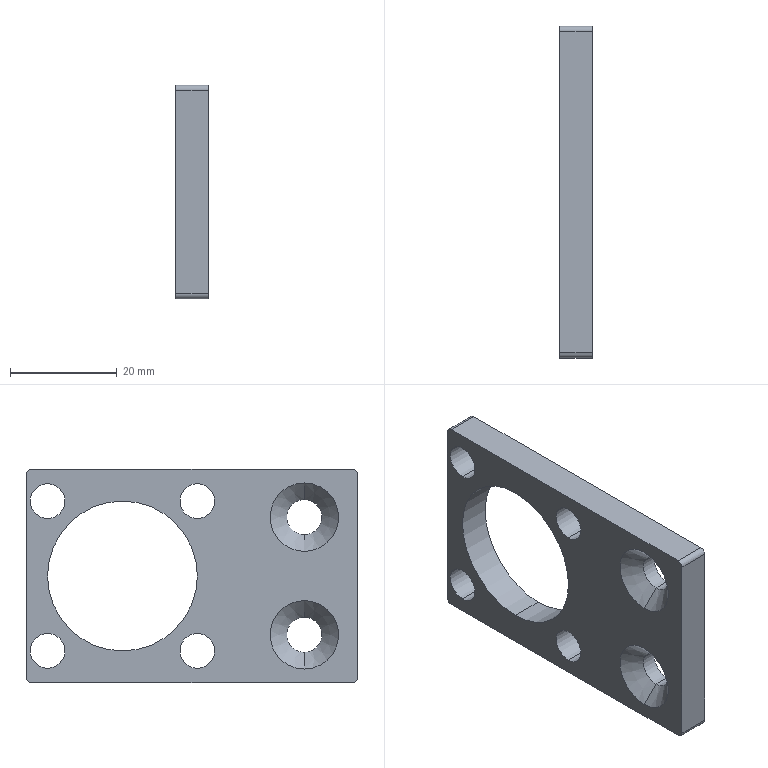Part | SolidWorks | features BaseBody 1 | 1 solid | 28 faces | box 6 x 62 x 40 mm | volume 9712 mm3 | cylinder 18 | plane 6 | cone 4 | commonest cylinder face diameters 6.5 x8 2 x4 6.6 x4 28 x2
STEP:
#1=CARTESIAN_POINT('',(6.,13.,14.));
#2=VERTEX_POINT('',#1);
#3=CARTESIAN_POINT('',(6.,13.,-14.));
#4=VERTEX_POINT('',#3);
#5=CARTESIAN_POINT('',(6.,13.,0.));
#6=DIRECTION('',(1.,0.,0.));
#7=DIRECTION('',(0.,0.,1.));
#8=AXIS2_PLACEMENT_3D('',#5,#6,#7);
#9=CIRCLE('',#8,14.);
#10=EDGE_CURVE('',#2,#4,#9,.T.);
#11=ORIENTED_EDGE('',*,*,#10,.T.);
#12=CARTESIAN_POINT('',(0.,13.,-14.));
#13=VERTEX_POINT('',#12);
#14=CARTESIAN_POINT('',(10.,13.,-14.));
#15=DIRECTION('',(-1.,0.,0.));
#16=VECTOR('',#15,1000.);
#17=LINE('',#14,#16);
#18=EDGE_CURVE('',#4,#13,#17,.T.);
#19=ORIENTED_EDGE('',*,*,#18,.T.);
#20=CARTESIAN_POINT('',(0.,13.,14.));
#21=VERTEX_POINT('',#20);
#22=CARTESIAN_POINT('',(0.,13.,0.));
#23=DIRECTION('',(1.,0.,0.));
#24=DIRECTION('',(0.,0.,1.));
#25=AXIS2_PLACEMENT_3D('',#22,#23,#24);
#26=CIRCLE('',#25,14.);
#27=EDGE_CURVE('',#21,#13,#26,.T.);
#28=ORIENTED_EDGE('',*,*,#27,.F.);
#29=CARTESIAN_POINT('',(10.,13.,14.));
#30=DIRECTION('',(-1.,0.,0.));
#31=VECTOR('',#30,1000.);
#32=LINE('',#29,#31);
#33=EDGE_CURVE('',#2,#21,#32,.T.);
#34=ORIENTED_EDGE('',*,*,#33,.F.);
#35=EDGE_LOOP('',(#11,#19,#28,#34));
#36=FACE_OUTER_BOUND('',#35,.T.);
#37=CARTESIAN_POINT('',(10.,13.,0.));
#38=DIRECTION('',(-1.,0.,0.));
#39=DIRECTION('',(0.,0.,1.));
#40=AXIS2_PLACEMENT_3D('',#37,#38,#39);
#41=CYLINDRICAL_SURFACE('',#40,14.);
#42=ADVANCED_FACE('',(#36),#41,.F.);
#43=CARTESIAN_POINT('',(6.,27.,-10.75));
#44=VERTEX_POINT('',#43);
#45=CARTESIAN_POINT('',(6.,27.,-17.25));
#46=VERTEX_POINT('',#45);
#47=CARTESIAN_POINT('',(6.,27.,-14.));
#48=DIRECTION('',(1.,0.,0.));
#49=DIRECTION('',(0.,0.,1.));
#50=AXIS2_PLACEMENT_3D('',#47,#48,#49);
#51=CIRCLE('',#50,3.25);
#52=EDGE_CURVE('',#44,#46,#51,.T.);
#53=ORIENTED_EDGE('',*,*,#52,.T.);
#54=CARTESIAN_POINT('',(0.,27.,-17.25));
#55=VERTEX_POINT('',#54);
#56=CARTESIAN_POINT('',(10.,27.,-17.25));
#57=DIRECTION('',(-1.,0.,0.));
#58=VECTOR('',#57,1000.);
#59=LINE('',#56,#58);
#60=EDGE_CURVE('',#46,#55,#59,.T.);
#61=ORIENTED_EDGE('',*,*,#60,.T.);
#62=CARTESIAN_POINT('',(0.,27.,-10.75));
#63=VERTEX_POINT('',#62);
#64=CARTESIAN_POINT('',(0.,27.,-14.));
#65=DIRECTION('',(1.,0.,0.));
#66=DIRECTION('',(0.,0.,1.));
#67=AXIS2_PLACEMENT_3D('',#64,#65,#66);
#68=CIRCLE('',#67,3.25);
#69=EDGE_CURVE('',#63,#55,#68,.T.);
#70=ORIENTED_EDGE('',*,*,#69,.F.);
#71=CARTESIAN_POINT('',(10.,27.,-10.75));
#72=DIRECTION('',(-1.,0.,0.));
#73=VECTOR('',#72,1000.);
#74=LINE('',#71,#73);
#75=EDGE_CURVE('',#44,#63,#74,.T.);
#76=ORIENTED_EDGE('',*,*,#75,.F.);
#77=EDGE_LOOP('',(#53,#61,#70,#76));
#78=FACE_OUTER_BOUND('',#77,.T.);
#79=CARTESIAN_POINT('',(10.,27.,-14.));
#80=DIRECTION('',(-1.,0.,0.));
#81=DIRECTION('',(0.,0.,1.));
#82=AXIS2_PLACEMENT_3D('',#79,#80,#81);
#83=CYLINDRICAL_SURFACE('',#82,3.25);
#84=ADVANCED_FACE('',(#78),#83,.F.);
#85=CARTESIAN_POINT('',(6.,-1.,-10.75));
#86=VERTEX_POINT('',#85);
#87=CARTESIAN_POINT('',(6.,-1.,-17.25));
#88=VERTEX_POINT('',#87);
#89=CARTESIAN_POINT('',(6.,-1.,-14.));
#90=DIRECTION('',(1.,0.,0.));
#91=DIRECTION('',(0.,0.,1.));
#92=AXIS2_PLACEMENT_3D('',#89,#90,#91);
#93=CIRCLE('',#92,3.25);
#94=EDGE_CURVE('',#86,#88,#93,.T.);
#95=ORIENTED_EDGE('',*,*,#94,.T.);
#96=CARTESIAN_POINT('',(0.,-1.,-17.25));
#97=VERTEX_POINT('',#96);
#98=CARTESIAN_POINT('',(10.,-1.,-17.25));
#99=DIRECTION('',(-1.,0.,0.));
#100=VECTOR('',#99,1000.);
#101=LINE('',#98,#100);
#102=EDGE_CURVE('',#88,#97,#101,.T.);
#103=ORIENTED_EDGE('',*,*,#102,.T.);
#104=CARTESIAN_POINT('',(0.,-1.,-10.75));
#105=VERTEX_POINT('',#104);
#106=CARTESIAN_POINT('',(0.,-1.,-14.));
#107=DIRECTION('',(1.,0.,0.));
#108=DIRECTION('',(0.,0.,1.));
#109=AXIS2_PLACEMENT_3D('',#106,#107,#108);
#110=CIRCLE('',#109,3.25);
#111=EDGE_CURVE('',#105,#97,#110,.T.);
#112=ORIENTED_EDGE('',*,*,#111,.F.);
#113=CARTESIAN_POINT('',(10.,-1.,-10.75));
#114=DIRECTION('',(-1.,0.,0.));
#115=VECTOR('',#114,1000.);
#116=LINE('',#113,#115);
#117=EDGE_CURVE('',#86,#105,#116,.T.);
#118=ORIENTED_EDGE('',*,*,#117,.F.);
#119=EDGE_LOOP('',(#95,#103,#112,#118));
#120=FACE_OUTER_BOUND('',#119,.T.);
#121=CARTESIAN_POINT('',(10.,-1.,-14.));
#122=DIRECTION('',(-1.,0.,0.));
#123=DIRECTION('',(0.,0.,1.));
#124=AXIS2_PLACEMENT_3D('',#121,#122,#123);
#125=CYLINDRICAL_SURFACE('',#124,3.25);
#126=ADVANCED_FACE('',(#120),#125,.F.);
#127=CARTESIAN_POINT('',(6.,-1.,17.25));
#128=VERTEX_POINT('',#127);
#129=CARTESIAN_POINT('',(6.,-1.,10.75));
#130=VERTEX_POINT('',#129);
#131=CARTESIAN_POINT('',(6.,-1.,14.));
#132=DIRECTION('',(1.,0.,0.));
#133=DIRECTION('',(0.,0.,1.));
#134=AXIS2_PLACEMENT_3D('',#131,#132,#133);
#135=CIRCLE('',#134,3.25);
#136=EDGE_CURVE('',#128,#130,#135,.T.);
#137=ORIENTED_EDGE('',*,*,#136,.T.);
#138=CARTESIAN_POINT('',(0.,-1.,10.75));
#139=VERTEX_POINT('',#138);
#140=CARTESIAN_POINT('',(10.,-1.,10.75));
#141=DIRECTION('',(-1.,0.,0.));
#142=VECTOR('',#141,1000.);
#143=LINE('',#140,#142);
#144=EDGE_CURVE('',#130,#139,#143,.T.);
#145=ORIENTED_EDGE('',*,*,#144,.T.);
#146=CARTESIAN_POINT('',(0.,-1.,17.25));
#147=VERTEX_POINT('',#146);
#148=CARTESIAN_POINT('',(0.,-1.,14.));
#149=DIRECTION('',(1.,0.,0.));
#150=DIRECTION('',(0.,0.,1.));
#151=AXIS2_PLACEMENT_3D('',#148,#149,#150);
#152=CIRCLE('',#151,3.25);
#153=EDGE_CURVE('',#147,#139,#152,.T.);
#154=ORIENTED_EDGE('',*,*,#153,.F.);
#155=CARTESIAN_POINT('',(10.,-1.,17.25));
#156=DIRECTION('',(-1.,0.,0.));
#157=VECTOR('',#156,1000.);
#158=LINE('',#155,#157);
#159=EDGE_CURVE('',#128,#147,#158,.T.);
#160=ORIENTED_EDGE('',*,*,#159,.F.);
#161=EDGE_LOOP('',(#137,#145,#154,#160));
#162=FACE_OUTER_BOUND('',#161,.T.);
#163=CARTESIAN_POINT('',(10.,-1.,14.));
#164=DIRECTION('',(-1.,0.,0.));
#165=DIRECTION('',(0.,0.,1.));
#166=AXIS2_PLACEMENT_3D('',#163,#164,#165);
#167=CYLINDRICAL_SURFACE('',#166,3.25);
#168=ADVANCED_FACE('',(#162),#167,.F.);
#169=CARTESIAN_POINT('',(6.,27.,17.25));
#170=VERTEX_POINT('',#169);
#171=CARTESIAN_POINT('',(6.,27.,10.75));
#172=VERTEX_POINT('',#171);
#173=CARTESIAN_POINT('',(6.,27.,14.));
#174=DIRECTION('',(1.,0.,0.));
#175=DIRECTION('',(0.,0.,1.));
#176=AXIS2_PLACEMENT_3D('',#173,#174,#175);
#177=CIRCLE('',#176,3.25);
#178=EDGE_CURVE('',#170,#172,#177,.T.);
#179=ORIENTED_EDGE('',*,*,#178,.T.);
#180=CARTESIAN_POINT('',(0.,27.,10.75));
#181=VERTEX_POINT('',#180);
#182=CARTESIAN_POINT('',(10.,27.,10.75));
#183=DIRECTION('',(-1.,0.,0.));
#184=VECTOR('',#183,1000.);
#185=LINE('',#182,#184);
#186=EDGE_CURVE('',#172,#181,#185,.T.);
#187=ORIENTED_EDGE('',*,*,#186,.T.);
#188=CARTESIAN_POINT('',(0.,27.,17.25));
#189=VERTEX_POINT('',#188);
#190=CARTESIAN_POINT('',(0.,27.,14.));
#191=DIRECTION('',(1.,0.,0.));
#192=DIRECTION('',(0.,0.,1.));
#193=AXIS2_PLACEMENT_3D('',#190,#191,#192);
#194=CIRCLE('',#193,3.25);
#195=EDGE_CURVE('',#189,#181,#194,.T.);
#196=ORIENTED_EDGE('',*,*,#195,.F.);
#197=CARTESIAN_POINT('',(10.,27.,17.25));
#198=DIRECTION('',(-1.,0.,0.));
#199=VECTOR('',#198,1000.);
#200=LINE('',#197,#199);
#201=EDGE_CURVE('',#170,#189,#200,.T.);
#202=ORIENTED_EDGE('',*,*,#201,.F.);
#203=EDGE_LOOP('',(#179,#187,#196,#202));
#204=FACE_OUTER_BOUND('',#203,.T.);
#205=CARTESIAN_POINT('',(10.,27.,14.));
#206=DIRECTION('',(-1.,0.,0.));
#207=DIRECTION('',(0.,0.,1.));
#208=AXIS2_PLACEMENT_3D('',#205,#206,#207);
#209=CYLINDRICAL_SURFACE('',#208,3.25);
#210=ADVANCED_FACE('',(#204),#209,.F.);
#211=CARTESIAN_POINT('',(6.,-21.,14.3));
#212=VERTEX_POINT('',#211);
#213=CARTESIAN_POINT('',(6.,-21.,7.7));
#214=VERTEX_POINT('',#213);
#215=CARTESIAN_POINT('',(6.,-21.,11.));
#216=DIRECTION('',(1.,0.,0.));
#217=DIRECTION('',(0.,0.,1.));
#218=AXIS2_PLACEMENT_3D('',#215,#216,#217);
#219=CIRCLE('',#218,3.3);
#220=EDGE_CURVE('',#212,#214,#219,.T.);
#221=ORIENTED_EDGE('',*,*,#220,.T.);
#222=CARTESIAN_POINT('',(3.1,-21.,7.7));
#223=VERTEX_POINT('',#222);
#224=CARTESIAN_POINT('',(0.,-21.,7.7));
#225=DIRECTION('',(-1.,0.,0.));
#226=VECTOR('',#225,1000.);
#227=LINE('',#224,#226);
#228=EDGE_CURVE('',#214,#223,#227,.T.);
#229=ORIENTED_EDGE('',*,*,#228,.T.);
#230=CARTESIAN_POINT('',(3.1,-21.,14.3));
#231=VERTEX_POINT('',#230);
#232=CARTESIAN_POINT('',(3.1,-21.,11.));
#233=DIRECTION('',(1.,0.,0.));
#234=DIRECTION('',(0.,0.,1.));
#235=AXIS2_PLACEMENT_3D('',#232,#233,#234);
#236=CIRCLE('',#235,3.3);
#237=EDGE_CURVE('',#231,#223,#236,.T.);
#238=ORIENTED_EDGE('',*,*,#237,.F.);
#239=CARTESIAN_POINT('',(0.,-21.,14.3));
#240=DIRECTION('',(-1.,0.,0.));
#241=VECTOR('',#240,1000.);
#242=LINE('',#239,#241);
#243=EDGE_CURVE('',#212,#231,#242,.T.);
#244=ORIENTED_EDGE('',*,*,#243,.F.);
#245=EDGE_LOOP('',(#221,#229,#238,#244));
#246=FACE_OUTER_BOUND('',#245,.T.);
#247=CARTESIAN_POINT('',(0.,-21.,11.));
#248=DIRECTION('',(-1.,0.,0.));
#249=DIRECTION('',(0.,0.,1.));
#250=AXIS2_PLACEMENT_3D('',#247,#248,#249);
#251=CYLINDRICAL_SURFACE('',#250,3.3);
#252=ADVANCED_FACE('',(#246),#251,.F.);
#253=CARTESIAN_POINT('',(6.,-21.,-7.7));
#254=VERTEX_POINT('',#253);
#255=CARTESIAN_POINT('',(6.,-21.,-14.3));
#256=VERTEX_POINT('',#255);
#257=CARTESIAN_POINT('',(6.,-21.,-11.));
#258=DIRECTION('',(1.,0.,0.));
#259=DIRECTION('',(0.,0.,1.));
#260=AXIS2_PLACEMENT_3D('',#257,#258,#259);
#261=CIRCLE('',#260,3.3);
#262=EDGE_CURVE('',#254,#256,#261,.T.);
#263=ORIENTED_EDGE('',*,*,#262,.T.);
#264=CARTESIAN_POINT('',(3.1,-21.,-14.3));
#265=VERTEX_POINT('',#264);
#266=CARTESIAN_POINT('',(0.,-21.,-14.3));
#267=DIRECTION('',(-1.,0.,0.));
#268=VECTOR('',#267,1000.);
#269=LINE('',#266,#268);
#270=EDGE_CURVE('',#256,#265,#269,.T.);
#271=ORIENTED_EDGE('',*,*,#270,.T.);
#272=CARTESIAN_POINT('',(3.1,-21.,-7.7));
#273=VERTEX_POINT('',#272);
#274=CARTESIAN_POINT('',(3.1,-21.,-11.));
#275=DIRECTION('',(1.,0.,0.));
#276=DIRECTION('',(0.,0.,1.));
#277=AXIS2_PLACEMENT_3D('',#274,#275,#276);
#278=CIRCLE('',#277,3.3);
#279=EDGE_CURVE('',#273,#265,#278,.T.);
#280=ORIENTED_EDGE('',*,*,#279,.F.);
#281=CARTESIAN_POINT('',(0.,-21.,-7.7));
#282=DIRECTION('',(-1.,0.,0.));
#283=VECTOR('',#282,1000.);
#284=LINE('',#281,#283);
#285=EDGE_CURVE('',#254,#273,#284,.T.);
#286=ORIENTED_EDGE('',*,*,#285,.F.);
#287=EDGE_LOOP('',(#263,#271,#280,#286));
#288=FACE_OUTER_BOUND('',#287,.T.);
#289=CARTESIAN_POINT('',(0.,-21.,-11.));
#290=DIRECTION('',(-1.,0.,0.));
#291=DIRECTION('',(0.,0.,1.));
#292=AXIS2_PLACEMENT_3D('',#289,#290,#291);
#293=CYLINDRICAL_SURFACE('',#292,3.3);
#294=ADVANCED_FACE('',(#288),#293,.F.);
#295=ORIENTED_EDGE('',*,*,#237,.T.);
#296=CARTESIAN_POINT('',(0.,-21.,4.6));
#297=VERTEX_POINT('',#296);
#298=CARTESIAN_POINT('',(0.,-21.,4.6));
#299=DIRECTION('',(-0.7071,0.,-0.7071));
#300=VECTOR('',#299,1000.);
#301=LINE('',#298,#300);
#302=EDGE_CURVE('',#223,#297,#301,.T.);
#303=ORIENTED_EDGE('',*,*,#302,.T.);
#304=CARTESIAN_POINT('',(0.,-21.,17.4));
#305=VERTEX_POINT('',#304);
#306=CARTESIAN_POINT('',(0.,-21.,11.));
#307=DIRECTION('',(1.,0.,0.));
#308=DIRECTION('',(0.,0.,1.));
#309=AXIS2_PLACEMENT_3D('',#306,#307,#308);
#310=CIRCLE('',#309,6.4);
#311=EDGE_CURVE('',#305,#297,#310,.T.);
#312=ORIENTED_EDGE('',*,*,#311,.F.);
#313=CARTESIAN_POINT('',(0.,-21.,17.4));
#314=DIRECTION('',(-0.7071,0.,0.7071));
#315=VECTOR('',#314,1000.);
#316=LINE('',#313,#315);
#317=EDGE_CURVE('',#231,#305,#316,.T.);
#318=ORIENTED_EDGE('',*,*,#317,.F.);
#319=EDGE_LOOP('',(#295,#303,#312,#318));
#320=FACE_OUTER_BOUND('',#319,.T.);
#321=CARTESIAN_POINT('',(0.,-21.,11.));
#322=DIRECTION('',(-1.,0.,0.));
#323=DIRECTION('',(0.,0.,1.));
#324=AXIS2_PLACEMENT_3D('',#321,#322,#323);
#325=CONICAL_SURFACE('',#324,6.4,0.7854);
#326=ADVANCED_FACE('',(#320),#325,.F.);
#327=ORIENTED_EDGE('',*,*,#279,.T.);
#328=CARTESIAN_POINT('',(0.,-21.,-17.4));
#329=VERTEX_POINT('',#328);
#330=CARTESIAN_POINT('',(0.,-21.,-17.4));
#331=DIRECTION('',(-0.7071,0.,-0.7071));
#332=VECTOR('',#331,1000.);
#333=LINE('',#330,#332);
#334=EDGE_CURVE('',#265,#329,#333,.T.);
#335=ORIENTED_EDGE('',*,*,#334,.T.);
#336=CARTESIAN_POINT('',(0.,-21.,-4.6));
#337=VERTEX_POINT('',#336);
#338=CARTESIAN_POINT('',(0.,-21.,-11.));
#339=DIRECTION('',(1.,0.,0.));
#340=DIRECTION('',(0.,0.,1.));
#341=AXIS2_PLACEMENT_3D('',#338,#339,#340);
#342=CIRCLE('',#341,6.4);
#343=EDGE_CURVE('',#337,#329,#342,.T.);
#344=ORIENTED_EDGE('',*,*,#343,.F.);
#345=CARTESIAN_POINT('',(0.,-21.,-4.6));
#346=DIRECTION('',(-0.7071,0.,0.7071));
#347=VECTOR('',#346,1000.);
#348=LINE('',#345,#347);
#349=EDGE_CURVE('',#273,#337,#348,.T.);
#350=ORIENTED_EDGE('',*,*,#349,.F.);
#351=EDGE_LOOP('',(#327,#335,#344,#350));
#352=FACE_OUTER_BOUND('',#351,.T.);
#353=CARTESIAN_POINT('',(0.,-21.,-11.));
#354=DIRECTION('',(-1.,0.,0.));
#355=DIRECTION('',(0.,0.,1.));
#356=AXIS2_PLACEMENT_3D('',#353,#354,#355);
#357=CONICAL_SURFACE('',#356,6.4,0.7854);
#358=ADVANCED_FACE('',(#352),#357,.F.);
#359=CARTESIAN_POINT('',(6.,-30.,-20.));
#360=VERTEX_POINT('',#359);
#361=CARTESIAN_POINT('',(6.,-31.,-19.));
#362=VERTEX_POINT('',#361);
#363=CARTESIAN_POINT('',(6.,-30.,-19.));
#364=DIRECTION('',(-1.,0.,0.));
#365=DIRECTION('',(0.,0.,1.));
#366=AXIS2_PLACEMENT_3D('',#363,#364,#365);
#367=CIRCLE('',#366,1.);
#368=EDGE_CURVE('',#360,#362,#367,.T.);
#369=ORIENTED_EDGE('',*,*,#368,.F.);
#370=CARTESIAN_POINT('',(6.,30.,-20.));
#371=VERTEX_POINT('',#370);
#372=CARTESIAN_POINT('',(6.,0.,-20.));
#373=DIRECTION('',(0.,-1.,0.));
#374=VECTOR('',#373,1000.);
#375=LINE('',#372,#374);
#376=EDGE_CURVE('',#371,#360,#375,.T.);
#377=ORIENTED_EDGE('',*,*,#376,.F.);
#378=CARTESIAN_POINT('',(6.,31.,-19.));
#379=VERTEX_POINT('',#378);
#380=CARTESIAN_POINT('',(6.,30.,-19.));
#381=DIRECTION('',(-1.,0.,0.));
#382=DIRECTION('',(0.,0.,1.));
#383=AXIS2_PLACEMENT_3D('',#380,#381,#382);
#384=CIRCLE('',#383,1.);
#385=EDGE_CURVE('',#379,#371,#384,.T.);
#386=ORIENTED_EDGE('',*,*,#385,.F.);
#387=CARTESIAN_POINT('',(6.,31.,19.));
#388=VERTEX_POINT('',#387);
#389=CARTESIAN_POINT('',(6.,31.,0.));
#390=DIRECTION('',(0.,0.,-1.));
#391=VECTOR('',#390,1000.);
#392=LINE('',#389,#391);
#393=EDGE_CURVE('',#388,#379,#392,.T.);
#394=ORIENTED_EDGE('',*,*,#393,.F.);
#395=CARTESIAN_POINT('',(6.,30.,20.));
#396=VERTEX_POINT('',#395);
#397=CARTESIAN_POINT('',(6.,30.,19.));
#398=DIRECTION('',(-1.,0.,0.));
#399=DIRECTION('',(0.,0.,1.));
#400=AXIS2_PLACEMENT_3D('',#397,#398,#399);
#401=CIRCLE('',#400,1.);
#402=EDGE_CURVE('',#396,#388,#401,.T.);
#403=ORIENTED_EDGE('',*,*,#402,.F.);
#404=CARTESIAN_POINT('',(6.,-30.,20.));
#405=VERTEX_POINT('',#404);
#406=CARTESIAN_POINT('',(6.,0.,20.));
#407=DIRECTION('',(0.,1.,0.));
#408=VECTOR('',#407,1000.);
#409=LINE('',#406,#408);
#410=EDGE_CURVE('',#405,#396,#409,.T.);
#411=ORIENTED_EDGE('',*,*,#410,.F.);
#412=CARTESIAN_POINT('',(6.,-31.,19.));
#413=VERTEX_POINT('',#412);
#414=CARTESIAN_POINT('',(6.,-30.,19.));
#415=DIRECTION('',(-1.,0.,0.));
#416=DIRECTION('',(0.,0.,1.));
#417=AXIS2_PLACEMENT_3D('',#414,#415,#416);
#418=CIRCLE('',#417,1.);
#419=EDGE_CURVE('',#413,#405,#418,.T.);
#420=ORIENTED_EDGE('',*,*,#419,.F.);
#421=CARTESIAN_POINT('',(6.,-31.,0.));
#422=DIRECTION('',(0.,0.,1.));
#423=VECTOR('',#422,1000.);
#424=LINE('',#421,#423);
#425=EDGE_CURVE('',#362,#413,#424,.T.);
#426=ORIENTED_EDGE('',*,*,#425,.F.);
#427=EDGE_LOOP('',(#369,#377,#386,#394,#403,#411,#420,#426));
#428=FACE_OUTER_BOUND('',#427,.T.);
#429=ORIENTED_EDGE('',*,*,#10,.F.);
#430=CARTESIAN_POINT('',(6.,13.,0.));
#431=DIRECTION('',(1.,0.,0.));
#432=DIRECTION('',(0.,0.,1.));
#433=AXIS2_PLACEMENT_3D('',#430,#431,#432);
#434=CIRCLE('',#433,14.);
#435=EDGE_CURVE('',#4,#2,#434,.T.);
#436=ORIENTED_EDGE('',*,*,#435,.F.);
#437=EDGE_LOOP('',(#429,#436));
#438=FACE_BOUND('',#437,.T.);
#439=ORIENTED_EDGE('',*,*,#52,.F.);
#440=CARTESIAN_POINT('',(6.,27.,-14.));
#441=DIRECTION('',(1.,0.,0.));
#442=DIRECTION('',(0.,0.,1.));
#443=AXIS2_PLACEMENT_3D('',#440,#441,#442);
#444=CIRCLE('',#443,3.25);
#445=EDGE_CURVE('',#46,#44,#444,.T.);
#446=ORIENTED_EDGE('',*,*,#445,.F.);
#447=EDGE_LOOP('',(#439,#446));
#448=FACE_BOUND('',#447,.T.);
#449=ORIENTED_EDGE('',*,*,#94,.F.);
#450=CARTESIAN_POINT('',(6.,-1.,-14.));
#451=DIRECTION('',(1.,0.,0.));
#452=DIRECTION('',(0.,0.,1.));
#453=AXIS2_PLACEMENT_3D('',#450,#451,#452);
#454=CIRCLE('',#453,3.25);
#455=EDGE_CURVE('',#88,#86,#454,.T.);
#456=ORIENTED_EDGE('',*,*,#455,.F.);
#457=EDGE_LOOP('',(#449,#456));
#458=FACE_BOUND('',#457,.T.);
#459=ORIENTED_EDGE('',*,*,#136,.F.);
#460=CARTESIAN_POINT('',(6.,-1.,14.));
#461=DIRECTION('',(1.,0.,0.));
#462=DIRECTION('',(0.,0.,1.));
#463=AXIS2_PLACEMENT_3D('',#460,#461,#462);
#464=CIRCLE('',#463,3.25);
#465=EDGE_CURVE('',#130,#128,#464,.T.);
#466=ORIENTED_EDGE('',*,*,#465,.F.);
#467=EDGE_LOOP('',(#459,#466));
#468=FACE_BOUND('',#467,.T.);
#469=ORIENTED_EDGE('',*,*,#178,.F.);
#470=CARTESIAN_POINT('',(6.,27.,14.));
#471=DIRECTION('',(1.,0.,0.));
#472=DIRECTION('',(0.,0.,1.));
#473=AXIS2_PLACEMENT_3D('',#470,#471,#472);
#474=CIRCLE('',#473,3.25);
#475=EDGE_CURVE('',#172,#170,#474,.T.);
#476=ORIENTED_EDGE('',*,*,#475,.F.);
#477=EDGE_LOOP('',(#469,#476));
#478=FACE_BOUND('',#477,.T.);
#479=ORIENTED_EDGE('',*,*,#220,.F.);
#480=CARTESIAN_POINT('',(6.,-21.,11.));
#481=DIRECTION('',(1.,0.,0.));
#482=DIRECTION('',(0.,0.,1.));
#483=AXIS2_PLACEMENT_3D('',#480,#481,#482);
#484=CIRCLE('',#483,3.3);
#485=EDGE_CURVE('',#214,#212,#484,.T.);
#486=ORIENTED_EDGE('',*,*,#485,.F.);
#487=EDGE_LOOP('',(#479,#486));
#488=FACE_BOUND('',#487,.T.);
#489=ORIENTED_EDGE('',*,*,#262,.F.);
#490=CARTESIAN_POINT('',(6.,-21.,-11.));
#491=DIRECTION('',(1.,0.,0.));
#492=DIRECTION('',(0.,0.,1.));
#493=AXIS2_PLACEMENT_3D('',#490,#491,#492);
#494=CIRCLE('',#493,3.3);
#495=EDGE_CURVE('',#256,#254,#494,.T.);
#496=ORIENTED_EDGE('',*,*,#495,.F.);
#497=EDGE_LOOP('',(#489,#496));
#498=FACE_BOUND('',#497,.T.);
#499=CARTESIAN_POINT('',(6.,0.,0.));
#500=DIRECTION('',(-1.,0.,0.));
#501=DIRECTION('',(0.,0.,1.));
#502=AXIS2_PLACEMENT_3D('',#499,#500,#501);
#503=PLANE('',#502);
#504=ADVANCED_FACE('',(#428,#438,#448,#458,#468,#478,#488,#498),#503,.F.);
#505=CARTESIAN_POINT('',(0.,-31.,-19.));
#506=VERTEX_POINT('',#505);
#507=CARTESIAN_POINT('',(6.,-31.,-19.));
#508=DIRECTION('',(-1.,0.,0.));
#509=VECTOR('',#508,1000.);
#510=LINE('',#507,#509);
#511=EDGE_CURVE('',#362,#506,#510,.T.);
#512=ORIENTED_EDGE('',*,*,#511,.F.);
#513=ORIENTED_EDGE('',*,*,#425,.T.);
#514=CARTESIAN_POINT('',(0.,-31.,19.));
#515=VERTEX_POINT('',#514);
#516=CARTESIAN_POINT('',(6.,-31.,19.));
#517=DIRECTION('',(1.,0.,0.));
#518=VECTOR('',#517,1000.);
#519=LINE('',#516,#518);
#520=EDGE_CURVE('',#515,#413,#519,.T.);
#521=ORIENTED_EDGE('',*,*,#520,.F.);
#522=CARTESIAN_POINT('',(0.,-31.,20.));
#523=DIRECTION('',(0.,0.,1.));
#524=VECTOR('',#523,1000.);
#525=LINE('',#522,#524);
#526=EDGE_CURVE('',#506,#515,#525,.T.);
#527=ORIENTED_EDGE('',*,*,#526,.F.);
#528=EDGE_LOOP('',(#512,#513,#521,#527));
#529=FACE_OUTER_BOUND('',#528,.T.);
#530=CARTESIAN_POINT('',(6.,-31.,20.));
#531=DIRECTION('',(0.,1.,0.));
#532=DIRECTION('',(0.,0.,1.));
#533=AXIS2_PLACEMENT_3D('',#530,#531,#532);
#534=PLANE('',#533);
#535=ADVANCED_FACE('',(#529),#534,.F.);
#536=CARTESIAN_POINT('',(0.,-30.,-20.));
#537=VERTEX_POINT('',#536);
#538=CARTESIAN_POINT('',(6.,-30.,-20.));
#539=DIRECTION('',(1.,0.,0.));
#540=VECTOR('',#539,1000.);
#541=LINE('',#538,#540);
#542=EDGE_CURVE('',#537,#360,#541,.T.);
#543=ORIENTED_EDGE('',*,*,#542,.F.);
#544=CARTESIAN_POINT('',(0.,30.,-20.));
#545=VERTEX_POINT('',#544);
#546=CARTESIAN_POINT('',(0.,-31.,-20.));
#547=DIRECTION('',(0.,-1.,0.));
#548=VECTOR('',#547,1000.);
#549=LINE('',#546,#548);
#550=EDGE_CURVE('',#545,#537,#549,.T.);
#551=ORIENTED_EDGE('',*,*,#550,.F.);
#552=CARTESIAN_POINT('',(6.,30.,-20.));
#553=DIRECTION('',(-1.,0.,0.));
#554=VECTOR('',#553,1000.);
#555=LINE('',#552,#554);
#556=EDGE_CURVE('',#371,#545,#555,.T.);
#557=ORIENTED_EDGE('',*,*,#556,.F.);
#558=ORIENTED_EDGE('',*,*,#376,.T.);
#559=EDGE_LOOP('',(#543,#551,#557,#558));
#560=FACE_OUTER_BOUND('',#559,.T.);
#561=CARTESIAN_POINT('',(6.,-31.,-20.));
#562=DIRECTION('',(0.,0.,1.));
#563=DIRECTION('',(1.,0.,0.));
#564=AXIS2_PLACEMENT_3D('',#561,#562,#563);
#565=PLANE('',#564);
#566=ADVANCED_FACE('',(#560),#565,.F.);
#567=CARTESIAN_POINT('',(0.,31.,-19.));
#568=VERTEX_POINT('',#567);
#569=CARTESIAN_POINT('',(6.,31.,-19.));
#570=DIRECTION('',(1.,0.,0.));
#571=VECTOR('',#570,1000.);
#572=LINE('',#569,#571);
#573=EDGE_CURVE('',#568,#379,#572,.T.);
#574=ORIENTED_EDGE('',*,*,#573,.F.);
#575=CARTESIAN_POINT('',(0.,31.,19.));
#576=VERTEX_POINT('',#575);
#577=CARTESIAN_POINT('',(0.,31.,20.));
#578=DIRECTION('',(0.,0.,-1.));
#579=VECTOR('',#578,1000.);
#580=LINE('',#577,#579);
#581=EDGE_CURVE('',#576,#568,#580,.T.);
#582=ORIENTED_EDGE('',*,*,#581,.F.);
#583=CARTESIAN_POINT('',(6.,31.,19.));
#584=DIRECTION('',(-1.,0.,0.));
#585=VECTOR('',#584,1000.);
#586=LINE('',#583,#585);
#587=EDGE_CURVE('',#388,#576,#586,.T.);
#588=ORIENTED_EDGE('',*,*,#587,.F.);
#589=ORIENTED_EDGE('',*,*,#393,.T.);
#590=EDGE_LOOP('',(#574,#582,#588,#589));
#591=FACE_OUTER_BOUND('',#590,.T.);
#592=CARTESIAN_POINT('',(6.,31.,20.));
#593=DIRECTION('',(0.,-1.,0.));
#594=DIRECTION('',(0.,0.,-1.));
#595=AXIS2_PLACEMENT_3D('',#592,#593,#594);
#596=PLANE('',#595);
#597=ADVANCED_FACE('',(#591),#596,.F.);
#598=CARTESIAN_POINT('',(0.,-30.,20.));
#599=VERTEX_POINT('',#598);
#600=CARTESIAN_POINT('',(6.,-30.,20.));
#601=DIRECTION('',(-1.,0.,0.));
#602=VECTOR('',#601,1000.);
#603=LINE('',#600,#602);
#604=EDGE_CURVE('',#405,#599,#603,.T.);
#605=ORIENTED_EDGE('',*,*,#604,.F.);
#606=ORIENTED_EDGE('',*,*,#410,.T.);
#607=CARTESIAN_POINT('',(0.,30.,20.));
#608=VERTEX_POINT('',#607);
#609=CARTESIAN_POINT('',(6.,30.,20.));
#610=DIRECTION('',(1.,0.,0.));
#611=VECTOR('',#610,1000.);
#612=LINE('',#609,#611);
#613=EDGE_CURVE('',#608,#396,#612,.T.);
#614=ORIENTED_EDGE('',*,*,#613,.F.);
#615=CARTESIAN_POINT('',(0.,-31.,20.));
#616=DIRECTION('',(0.,1.,0.));
#617=VECTOR('',#616,1000.);
#618=LINE('',#615,#617);
#619=EDGE_CURVE('',#599,#608,#618,.T.);
#620=ORIENTED_EDGE('',*,*,#619,.F.);
#621=EDGE_LOOP('',(#605,#606,#614,#620));
#622=FACE_OUTER_BOUND('',#621,.T.);
#623=CARTESIAN_POINT('',(6.,-31.,20.));
#624=DIRECTION('',(0.,0.,-1.));
#625=DIRECTION('',(-1.,0.,0.));
#626=AXIS2_PLACEMENT_3D('',#623,#624,#625);
#627=PLANE('',#626);
#628=ADVANCED_FACE('',(#622),#627,.F.);
#629=ORIENTED_EDGE('',*,*,#18,.F.);
#630=ORIENTED_EDGE('',*,*,#435,.T.);
#631=ORIENTED_EDGE('',*,*,#33,.T.);
#632=CARTESIAN_POINT('',(0.,13.,0.));
#633=DIRECTION('',(1.,0.,0.));
#634=DIRECTION('',(0.,0.,1.));
#635=AXIS2_PLACEMENT_3D('',#632,#633,#634);
#636=CIRCLE('',#635,14.);
#637=EDGE_CURVE('',#13,#21,#636,.T.);
#638=ORIENTED_EDGE('',*,*,#637,.F.);
#639=EDGE_LOOP('',(#629,#630,#631,#638));
#640=FACE_OUTER_BOUND('',#639,.T.);
#641=CARTESIAN_POINT('',(10.,13.,0.));
#642=DIRECTION('',(-1.,0.,0.));
#643=DIRECTION('',(0.,0.,1.));
#644=AXIS2_PLACEMENT_3D('',#641,#642,#643);
#645=CYLINDRICAL_SURFACE('',#644,14.);
#646=ADVANCED_FACE('',(#640),#645,.F.);
#647=ORIENTED_EDGE('',*,*,#60,.F.);
#648=ORIENTED_EDGE('',*,*,#445,.T.);
#649=ORIENTED_EDGE('',*,*,#75,.T.);
#650=CARTESIAN_POINT('',(0.,27.,-14.));
#651=DIRECTION('',(1.,0.,0.));
#652=DIRECTION('',(0.,0.,1.));
#653=AXIS2_PLACEMENT_3D('',#650,#651,#652);
#654=CIRCLE('',#653,3.25);
#655=EDGE_CURVE('',#55,#63,#654,.T.);
#656=ORIENTED_EDGE('',*,*,#655,.F.);
#657=EDGE_LOOP('',(#647,#648,#649,#656));
#658=FACE_OUTER_BOUND('',#657,.T.);
#659=CARTESIAN_POINT('',(10.,27.,-14.));
#660=DIRECTION('',(-1.,0.,0.));
#661=DIRECTION('',(0.,0.,1.));
#662=AXIS2_PLACEMENT_3D('',#659,#660,#661);
#663=CYLINDRICAL_SURFACE('',#662,3.25);
#664=ADVANCED_FACE('',(#658),#663,.F.);
#665=ORIENTED_EDGE('',*,*,#102,.F.);
#666=ORIENTED_EDGE('',*,*,#455,.T.);
#667=ORIENTED_EDGE('',*,*,#117,.T.);
#668=CARTESIAN_POINT('',(0.,-1.,-14.));
#669=DIRECTION('',(1.,0.,0.));
#670=DIRECTION('',(0.,0.,1.));
#671=AXIS2_PLACEMENT_3D('',#668,#669,#670);
#672=CIRCLE('',#671,3.25);
#673=EDGE_CURVE('',#97,#105,#672,.T.);
#674=ORIENTED_EDGE('',*,*,#673,.F.);
#675=EDGE_LOOP('',(#665,#666,#667,#674));
#676=FACE_OUTER_BOUND('',#675,.T.);
#677=CARTESIAN_POINT('',(10.,-1.,-14.));
#678=DIRECTION('',(-1.,0.,0.));
#679=DIRECTION('',(0.,0.,1.));
#680=AXIS2_PLACEMENT_3D('',#677,#678,#679);
#681=CYLINDRICAL_SURFACE('',#680,3.25);
#682=ADVANCED_FACE('',(#676),#681,.F.);
#683=ORIENTED_EDGE('',*,*,#144,.F.);
#684=ORIENTED_EDGE('',*,*,#465,.T.);
#685=ORIENTED_EDGE('',*,*,#159,.T.);
#686=CARTESIAN_POINT('',(0.,-1.,14.));
#687=DIRECTION('',(1.,0.,0.));
#688=DIRECTION('',(0.,0.,1.));
#689=AXIS2_PLACEMENT_3D('',#686,#687,#688);
#690=CIRCLE('',#689,3.25);
#691=EDGE_CURVE('',#139,#147,#690,.T.);
#692=ORIENTED_EDGE('',*,*,#691,.F.);
#693=EDGE_LOOP('',(#683,#684,#685,#692));
#694=FACE_OUTER_BOUND('',#693,.T.);
#695=CARTESIAN_POINT('',(10.,-1.,14.));
#696=DIRECTION('',(-1.,0.,0.));
#697=DIRECTION('',(0.,0.,1.));
#698=AXIS2_PLACEMENT_3D('',#695,#696,#697);
#699=CYLINDRICAL_SURFACE('',#698,3.25);
#700=ADVANCED_FACE('',(#694),#699,.F.);
#701=ORIENTED_EDGE('',*,*,#186,.F.);
#702=ORIENTED_EDGE('',*,*,#475,.T.);
#703=ORIENTED_EDGE('',*,*,#201,.T.);
#704=CARTESIAN_POINT('',(0.,27.,14.));
#705=DIRECTION('',(1.,0.,0.));
#706=DIRECTION('',(0.,0.,1.));
#707=AXIS2_PLACEMENT_3D('',#704,#705,#706);
#708=CIRCLE('',#707,3.25);
#709=EDGE_CURVE('',#181,#189,#708,.T.);
#710=ORIENTED_EDGE('',*,*,#709,.F.);
#711=EDGE_LOOP('',(#701,#702,#703,#710));
#712=FACE_OUTER_BOUND('',#711,.T.);
#713=CARTESIAN_POINT('',(10.,27.,14.));
#714=DIRECTION('',(-1.,0.,0.));
#715=DIRECTION('',(0.,0.,1.));
#716=AXIS2_PLACEMENT_3D('',#713,#714,#715);
#717=CYLINDRICAL_SURFACE('',#716,3.25);
#718=ADVANCED_FACE('',(#712),#717,.F.);
#719=ORIENTED_EDGE('',*,*,#228,.F.);
#720=ORIENTED_EDGE('',*,*,#485,.T.);
#721=ORIENTED_EDGE('',*,*,#243,.T.);
#722=CARTESIAN_POINT('',(3.1,-21.,11.));
#723=DIRECTION('',(1.,0.,0.));
#724=DIRECTION('',(0.,0.,1.));
#725=AXIS2_PLACEMENT_3D('',#722,#723,#724);
#726=CIRCLE('',#725,3.3);
#727=EDGE_CURVE('',#223,#231,#726,.T.);
#728=ORIENTED_EDGE('',*,*,#727,.F.);
#729=EDGE_LOOP('',(#719,#720,#721,#728));
#730=FACE_OUTER_BOUND('',#729,.T.);
#731=CARTESIAN_POINT('',(0.,-21.,11.));
#732=DIRECTION('',(-1.,0.,0.));
#733=DIRECTION('',(0.,0.,1.));
#734=AXIS2_PLACEMENT_3D('',#731,#732,#733);
#735=CYLINDRICAL_SURFACE('',#734,3.3);
#736=ADVANCED_FACE('',(#730),#735,.F.);
#737=ORIENTED_EDGE('',*,*,#270,.F.);
#738=ORIENTED_EDGE('',*,*,#495,.T.);
#739=ORIENTED_EDGE('',*,*,#285,.T.);
#740=CARTESIAN_POINT('',(3.1,-21.,-11.));
#741=DIRECTION('',(1.,0.,0.));
#742=DIRECTION('',(0.,0.,1.));
#743=AXIS2_PLACEMENT_3D('',#740,#741,#742);
#744=CIRCLE('',#743,3.3);
#745=EDGE_CURVE('',#265,#273,#744,.T.);
#746=ORIENTED_EDGE('',*,*,#745,.F.);
#747=EDGE_LOOP('',(#737,#738,#739,#746));
#748=FACE_OUTER_BOUND('',#747,.T.);
#749=CARTESIAN_POINT('',(0.,-21.,-11.));
#750=DIRECTION('',(-1.,0.,0.));
#751=DIRECTION('',(0.,0.,1.));
#752=AXIS2_PLACEMENT_3D('',#749,#750,#751);
#753=CYLINDRICAL_SURFACE('',#752,3.3);
#754=ADVANCED_FACE('',(#748),#753,.F.);
#755=ORIENTED_EDGE('',*,*,#581,.T.);
#756=CARTESIAN_POINT('',(0.,30.,-19.));
#757=DIRECTION('',(-1.,0.,0.));
#758=DIRECTION('',(0.,0.,1.));
#759=AXIS2_PLACEMENT_3D('',#756,#757,#758);
#760=CIRCLE('',#759,1.);
#761=EDGE_CURVE('',#568,#545,#760,.T.);
#762=ORIENTED_EDGE('',*,*,#761,.T.);
#763=ORIENTED_EDGE('',*,*,#550,.T.);
#764=CARTESIAN_POINT('',(0.,-30.,-19.));
#765=DIRECTION('',(-1.,0.,0.));
#766=DIRECTION('',(0.,0.,1.));
#767=AXIS2_PLACEMENT_3D('',#764,#765,#766);
#768=CIRCLE('',#767,1.);
#769=EDGE_CURVE('',#537,#506,#768,.T.);
#770=ORIENTED_EDGE('',*,*,#769,.T.);
#771=ORIENTED_EDGE('',*,*,#526,.T.);
#772=CARTESIAN_POINT('',(0.,-30.,19.));
#773=DIRECTION('',(-1.,0.,0.));
#774=DIRECTION('',(0.,0.,1.));
#775=AXIS2_PLACEMENT_3D('',#772,#773,#774);
#776=CIRCLE('',#775,1.);
#777=EDGE_CURVE('',#515,#599,#776,.T.);
#778=ORIENTED_EDGE('',*,*,#777,.T.);
#779=ORIENTED_EDGE('',*,*,#619,.T.);
#780=CARTESIAN_POINT('',(0.,30.,19.));
#781=DIRECTION('',(-1.,0.,0.));
#782=DIRECTION('',(0.,0.,1.));
#783=AXIS2_PLACEMENT_3D('',#780,#781,#782);
#784=CIRCLE('',#783,1.);
#785=EDGE_CURVE('',#608,#576,#784,.T.);
#786=ORIENTED_EDGE('',*,*,#785,.T.);
#787=EDGE_LOOP('',(#755,#762,#763,#770,#771,#778,#779,#786));
#788=FACE_OUTER_BOUND('',#787,.T.);
#789=ORIENTED_EDGE('',*,*,#27,.T.);
#790=ORIENTED_EDGE('',*,*,#637,.T.);
#791=EDGE_LOOP('',(#789,#790));
#792=FACE_BOUND('',#791,.T.);
#793=ORIENTED_EDGE('',*,*,#69,.T.);
#794=ORIENTED_EDGE('',*,*,#655,.T.);
#795=EDGE_LOOP('',(#793,#794));
#796=FACE_BOUND('',#795,.T.);
#797=ORIENTED_EDGE('',*,*,#111,.T.);
#798=ORIENTED_EDGE('',*,*,#673,.T.);
#799=EDGE_LOOP('',(#797,#798));
#800=FACE_BOUND('',#799,.T.);
#801=ORIENTED_EDGE('',*,*,#153,.T.);
#802=ORIENTED_EDGE('',*,*,#691,.T.);
#803=EDGE_LOOP('',(#801,#802));
#804=FACE_BOUND('',#803,.T.);
#805=ORIENTED_EDGE('',*,*,#195,.T.);
#806=ORIENTED_EDGE('',*,*,#709,.T.);
#807=EDGE_LOOP('',(#805,#806));
#808=FACE_BOUND('',#807,.T.);
#809=ORIENTED_EDGE('',*,*,#311,.T.);
#810=CARTESIAN_POINT('',(0.,-21.,11.));
#811=DIRECTION('',(1.,0.,0.));
#812=DIRECTION('',(0.,0.,1.));
#813=AXIS2_PLACEMENT_3D('',#810,#811,#812);
#814=CIRCLE('',#813,6.4);
#815=EDGE_CURVE('',#297,#305,#814,.T.);
#816=ORIENTED_EDGE('',*,*,#815,.T.);
#817=EDGE_LOOP('',(#809,#816));
#818=FACE_BOUND('',#817,.T.);
#819=ORIENTED_EDGE('',*,*,#343,.T.);
#820=CARTESIAN_POINT('',(0.,-21.,-11.));
#821=DIRECTION('',(1.,0.,0.));
#822=DIRECTION('',(0.,0.,1.));
#823=AXIS2_PLACEMENT_3D('',#820,#821,#822);
#824=CIRCLE('',#823,6.4);
#825=EDGE_CURVE('',#329,#337,#824,.T.);
#826=ORIENTED_EDGE('',*,*,#825,.T.);
#827=EDGE_LOOP('',(#819,#826));
#828=FACE_BOUND('',#827,.T.);
#829=CARTESIAN_POINT('',(0.,0.,0.));
#830=DIRECTION('',(-1.,0.,0.));
#831=DIRECTION('',(0.,0.,1.));
#832=AXIS2_PLACEMENT_3D('',#829,#830,#831);
#833=PLANE('',#832);
#834=ADVANCED_FACE('',(#788,#792,#796,#800,#804,#808,#818,#828),#833,.T.);
#835=ORIENTED_EDGE('',*,*,#769,.F.);
#836=ORIENTED_EDGE('',*,*,#542,.T.);
#837=ORIENTED_EDGE('',*,*,#368,.T.);
#838=ORIENTED_EDGE('',*,*,#511,.T.);
#839=EDGE_LOOP('',(#835,#836,#837,#838));
#840=FACE_OUTER_BOUND('',#839,.T.);
#841=CARTESIAN_POINT('',(6.,-30.,-19.));
#842=DIRECTION('',(-1.,0.,0.));
#843=DIRECTION('',(0.,0.,1.));
#844=AXIS2_PLACEMENT_3D('',#841,#842,#843);
#845=CYLINDRICAL_SURFACE('',#844,1.);
#846=ADVANCED_FACE('',(#840),#845,.T.);
#847=ORIENTED_EDGE('',*,*,#777,.F.);
#848=ORIENTED_EDGE('',*,*,#520,.T.);
#849=ORIENTED_EDGE('',*,*,#419,.T.);
#850=ORIENTED_EDGE('',*,*,#604,.T.);
#851=EDGE_LOOP('',(#847,#848,#849,#850));
#852=FACE_OUTER_BOUND('',#851,.T.);
#853=CARTESIAN_POINT('',(6.,-30.,19.));
#854=DIRECTION('',(-1.,0.,0.));
#855=DIRECTION('',(0.,0.,1.));
#856=AXIS2_PLACEMENT_3D('',#853,#854,#855);
#857=CYLINDRICAL_SURFACE('',#856,1.);
#858=ADVANCED_FACE('',(#852),#857,.T.);
#859=ORIENTED_EDGE('',*,*,#761,.F.);
#860=ORIENTED_EDGE('',*,*,#573,.T.);
#861=ORIENTED_EDGE('',*,*,#385,.T.);
#862=ORIENTED_EDGE('',*,*,#556,.T.);
#863=EDGE_LOOP('',(#859,#860,#861,#862));
#864=FACE_OUTER_BOUND('',#863,.T.);
#865=CARTESIAN_POINT('',(6.,30.,-19.));
#866=DIRECTION('',(-1.,0.,0.));
#867=DIRECTION('',(0.,0.,1.));
#868=AXIS2_PLACEMENT_3D('',#865,#866,#867);
#869=CYLINDRICAL_SURFACE('',#868,1.);
#870=ADVANCED_FACE('',(#864),#869,.T.);
#871=ORIENTED_EDGE('',*,*,#785,.F.);
#872=ORIENTED_EDGE('',*,*,#613,.T.);
#873=ORIENTED_EDGE('',*,*,#402,.T.);
#874=ORIENTED_EDGE('',*,*,#587,.T.);
#875=EDGE_LOOP('',(#871,#872,#873,#874));
#876=FACE_OUTER_BOUND('',#875,.T.);
#877=CARTESIAN_POINT('',(6.,30.,19.));
#878=DIRECTION('',(-1.,0.,0.));
#879=DIRECTION('',(0.,0.,1.));
#880=AXIS2_PLACEMENT_3D('',#877,#878,#879);
#881=CYLINDRICAL_SURFACE('',#880,1.);
#882=ADVANCED_FACE('',(#876),#881,.T.);
#883=ORIENTED_EDGE('',*,*,#302,.F.);
#884=ORIENTED_EDGE('',*,*,#727,.T.);
#885=ORIENTED_EDGE('',*,*,#317,.T.);
#886=ORIENTED_EDGE('',*,*,#815,.F.);
#887=EDGE_LOOP('',(#883,#884,#885,#886));
#888=FACE_OUTER_BOUND('',#887,.T.);
#889=CARTESIAN_POINT('',(0.,-21.,11.));
#890=DIRECTION('',(-1.,0.,0.));
#891=DIRECTION('',(0.,0.,1.));
#892=AXIS2_PLACEMENT_3D('',#889,#890,#891);
#893=CONICAL_SURFACE('',#892,6.4,0.7854);
#894=ADVANCED_FACE('',(#888),#893,.F.);
#895=ORIENTED_EDGE('',*,*,#334,.F.);
#896=ORIENTED_EDGE('',*,*,#745,.T.);
#897=ORIENTED_EDGE('',*,*,#349,.T.);
#898=ORIENTED_EDGE('',*,*,#825,.F.);
#899=EDGE_LOOP('',(#895,#896,#897,#898));
#900=FACE_OUTER_BOUND('',#899,.T.);
#901=CARTESIAN_POINT('',(0.,-21.,-11.));
#902=DIRECTION('',(-1.,0.,0.));
#903=DIRECTION('',(0.,0.,1.));
#904=AXIS2_PLACEMENT_3D('',#901,#902,#903);
#905=CONICAL_SURFACE('',#904,6.4,0.7854);
#906=ADVANCED_FACE('',(#900),#905,.F.);
#907=CLOSED_SHELL('',(#42,#84,#126,#168,#210,#252,#294,#326,#358,#504,#535,#566,#597,#628,#646,#664,#682,#700,#718,#736,#754,#834,#846,#858,#870,#882,#894,#906));
#908=MANIFOLD_SOLID_BREP('',#907);
#909=CARTESIAN_POINT('',(0.,0.,0.));
#910=DIRECTION('',(0.,0.,1.));
#911=DIRECTION('',(1.,0.,0.));
#912=AXIS2_PLACEMENT_3D('',#909,#910,#911);
#913=(LENGTH_UNIT()NAMED_UNIT(*)SI_UNIT(.MILLI.,.METRE.));
#914=UNCERTAINTY_MEASURE_WITH_UNIT(LENGTH_MEASURE(0.00001),#913,'','');
#915=(NAMED_UNIT(*)PLANE_ANGLE_UNIT()SI_UNIT($,.RADIAN.));
#916=(NAMED_UNIT(*)SI_UNIT($,.STERADIAN.)SOLID_ANGLE_UNIT());
#917=(GEOMETRIC_REPRESENTATION_CONTEXT(3)GLOBAL_UNCERTAINTY_ASSIGNED_CONTEXT((#914))GLOBAL_UNIT_ASSIGNED_CONTEXT((#913,#915,#916))REPRESENTATION_CONTEXT('',''));
#918=ADVANCED_BREP_SHAPE_REPRESENTATION('',(#908,#912),#917);